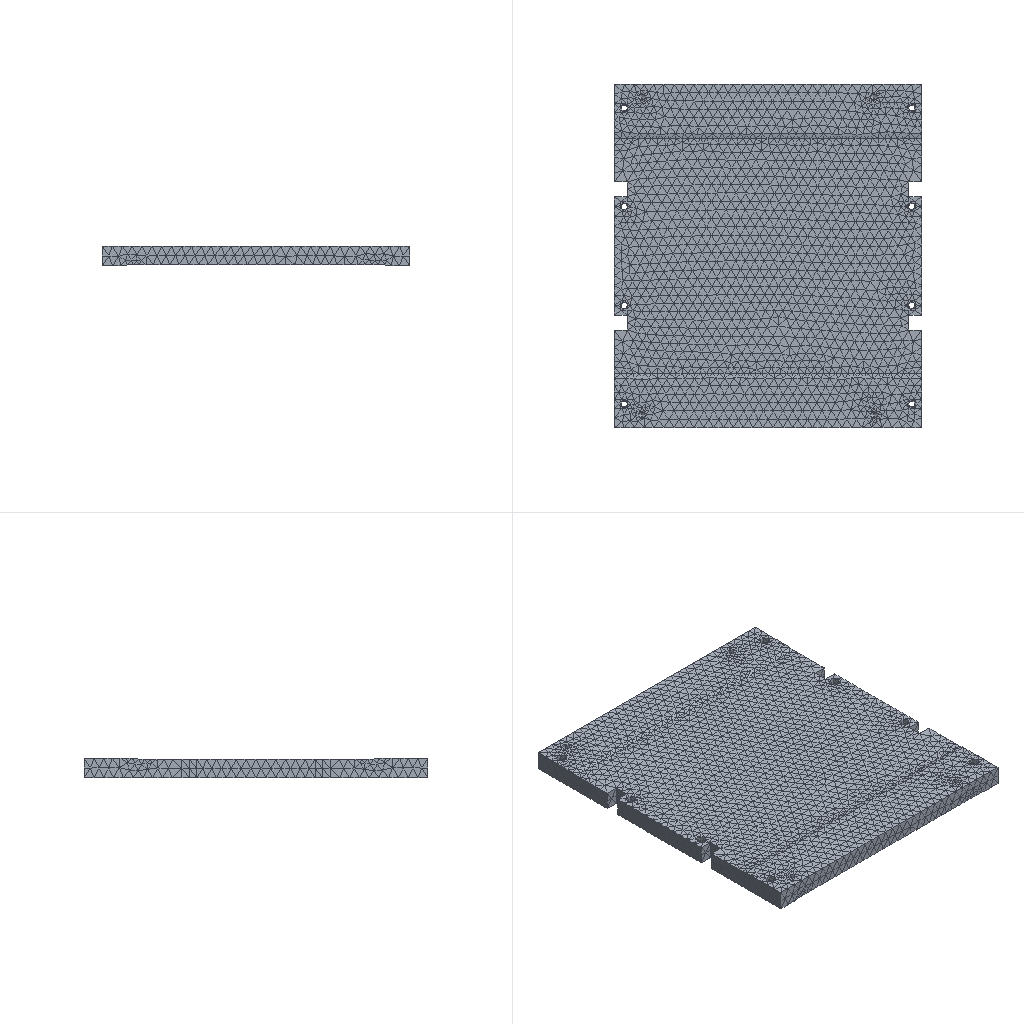Simulation study | nx simcenter
Set-up summary:
category,name,step,type,value,unit,region
solver,nx_nastran (Simcenter)
units,not stated in the deck,,not stated
analysis,deck,,static,static
analysis,solution,,SOL,101
load_step,SUBCASE 1,1,SUBCASE,SPC=1 LOAD=2
load_step,requested,,,1
mesh,nodes,,,32449
mesh,elements,,,16825
element_type,CTETRA,,solid,16825
load,nodal force total,,FX,0.0,model units
load,nodal force total,,FY,0.0,model units
load,nodal force total,,FZ,-1000000.003,model units
load,load commands in deck,,count,1838
bc,support commands in deck,,count,1468
analysis,NX solution 0,,Structural,Linear Statics - Single Constraint
check,setup vs results,,match,every grid point's frame and coordinates and every element id; grid points of CTETRA elements
Nastran input file, long lists of numbers shortened:
$*$$$$$$$$$$$$$$$$$$$$$$$$$$$$$$$$$$$$$$$$$$$$$$$$$$$$$$$$$$$$$$$$$
$*
$*                    NX v10.0.0.24 TRANSLATOR
$*                    FOR NX NASTRAN VERSION 10.0
$ (33 more lines like these left out)
ASSIGN OUTPUT2='101_sim1-solution_1.op2' UNIT=12
$*
$*$$$$$$$$$$$$$$$$$$$$$$$$$$$$$$$$$$$
$*
$* EXECUTIVE CONTROL
$*
$*$$$$$$$$$$$$$$$$$$$$$$$$$$$$$$$$$$$
$*
ID,NASTRAN,101_sim1-solution_1
SOL 101
CEND
$*
$*$$$$$$$$$$$$$$$$$$$$$$$$$$$$$$$$$$$
$*
$* CASE CONTROL
$*
$*$$$$$$$$$$$$$$$$$$$$$$$$$$$$$$$$$$$
$*
TITLE = Solution 1
ECHO = NONE
SPC = 1
OUTPUT
BCRESULTS(TRACTION,FORCE,PLOT) = ALL
DISPLACEMENT(PLOT) = ALL
ESE(PLOT) = ALL
FORCE(PLOT,CORNER) = ALL
OLOAD(PLOT) = ALL
SPCFORCES(PLOT) = ALL
STRAIN(PLOT,FIBER,CORNER) = ALL
STRESS(PLOT,CORNER) = ALL
$*  NX Step: Subcase - Static Loads 1
SUBCASE 1
LABEL = Subcase - Static Loads 1
LOAD = 2
$*
$*$$$$$$$$$$$$$$$$$$$$$$$$$$$$$$$$$$$
$*
$* BULK DATA
$*
$*$$$$$$$$$$$$$$$$$$$$$$$$$$$$$$$$$$$
$*
BEGIN BULK
$*
$* PARAM CARDS
$*
PARAM      K6ROT100.0000
PARAM     OIBULK     YES
PARAM    OMACHPR     YES
PARAM       POST      -2
PARAM    POSTEXT     YES
PARAM    UNITSYS   MN-MM
$*
$* GRID CARDS
$*
GRID*              32266               0-1.555000000E+02-1.740000000E+02+
*       2.0000000000E+01               0
GRID*              32267               0-1.555000000E+02-1.740000000E+02+
*       0.0000000000E+00               0
$ (64894 more lines like these left out)
$*
$* ELEMENT CARDS
$*
$*  NX Mesh Collector: Solid(1)
$*  NX Mesh: 3d_mesh(1)
CTETRA         1       1       1   18567   19310   19257     445   22055+
+            446     447   22054   22056
CTETRA         2       1       1       2   16326       3     448     449+
+            450     451     452     453
$ (33646 more lines like these left out)
$*
$* PROPERTY CARDS
$*
$*  NX Property: PSOLID1
PSOLID         1       1       0                           SMECH
$*
$* MATERIAL CARDS
$*
$*  NX Material: 2A12
MAT1           17.3119+7        0.3300002.8000-62.1355-5
MATT1          1       1               2               3
TABLEM1        1                                                        +
+        20.00007.3119+7 21.11007.3119+7 23.89007.3119+7 37.78007.3119+7+
+        51.67007.3119+7 65.56007.2429+7 79.44007.2429+7 93.33007.1739+7+
+       107.22007.1049+7121.11007.0359+7135.00006.9670+7148.89006.8980+7+
+       162.78006.8290+7176.67006.6910+7190.56006.6221+7204.44006.4841+7+
+       218.33006.3461+7232.22006.1392+7246.11006.0012+7260.00005.8633+7+
+       273.89005.7253+7287.78005.5184+7301.67005.3804+7315.56005.1735+7+
+       329.44004.9665+7343.33004.7596+7357.22004.6216+7371.11004.4147+7+
+           ENDT
TABLEM1        2                                                        +
+        20.00000.330000 21.11000.330000    ENDT
TABLEM1        3                                                        +
+        20.00002.1600-5 93.33002.2500-5107.22002.2662-5121.11002.2824-5+
+       135.00002.2968-5148.89002.3130-5162.78002.3274-5176.67002.3418-5+
+       190.56002.3544-5204.44002.3688-5218.33002.3814-5232.22002.3958-5+
+       246.11002.4066-5260.00002.4192-5273.89002.4300-5287.78002.4408-5+
+       301.67002.4498-5315.56002.4606-5329.44002.4696-5343.33002.4786-5+
+       357.22002.4876-5371.11002.4984-5385.00002.5110-5398.89002.5254-5+
+       412.78002.5398-5426.67002.5560-5    ENDT
$*
$* LOAD AND CONSTRAINT CARDS
$*
$*  NX Load and Constraint: Fixed(1)
SPC            1   25448  123456  0.0000
SPC            1   25449  123456  0.0000
SPC            1   25450  123456  0.0000
SPC            1   25451  123456  0.0000
$ (1464 more lines like these left out)
$*  NX Load and Constraint: Force(1)
FORCE          2   27091       0647.0852  0.0000  0.0000-1.00000
FORCE          2   27092       0631.5479  0.0000  0.0000-1.00000
FORCE          2   27093       0689.1535  0.0000  0.0000-1.00000
FORCE          2   27094       0579.7995  0.0000  0.0000-1.00000
$ (1834 more lines like these left out)
ENDDATA 220f11fd
Results summary:
result,analysis,,,static
result,last_loadstep,,,1
result,primary field,,,displacements
result,max displacement,,,0.01187,model units
result,reaction total,,FX,-0.2141,model units
result,reaction total,,FY,0.03809,model units
result,reaction total,,FZ,999999.438,model units
result,NX solution 0,,loadcases,1,mm